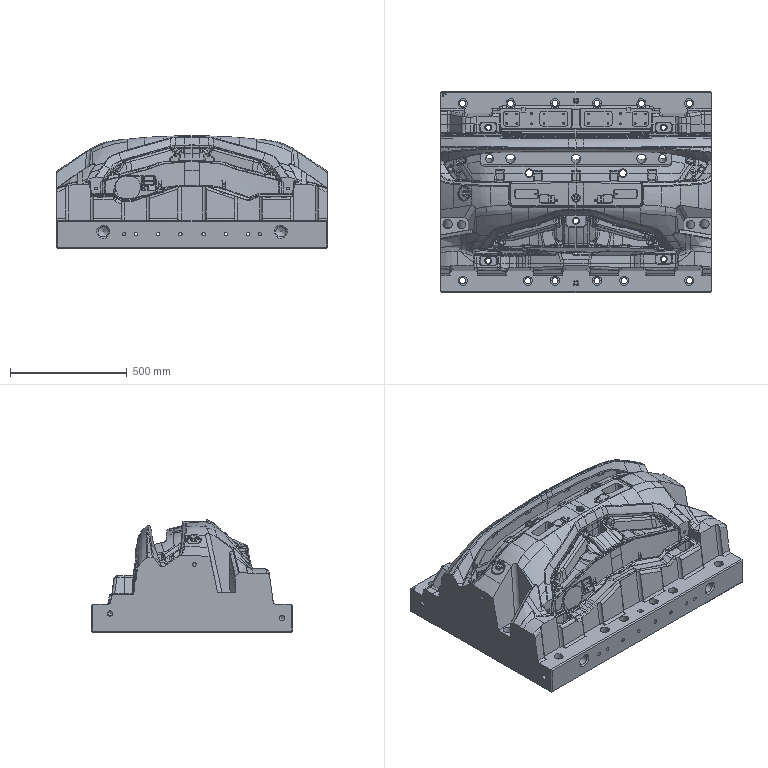Part | STEP file | solid 122 | 1 solid | 3004 faces | volume 271064204 mm3 | spline 1928 | cylinder 463 | plane 437 | cone 100 | other 57 | sphere 19 | commonest cylinder face diameters 15 x96 26 x85 30.5 x36 6.8 x18 1.013 x16 11.143 x16